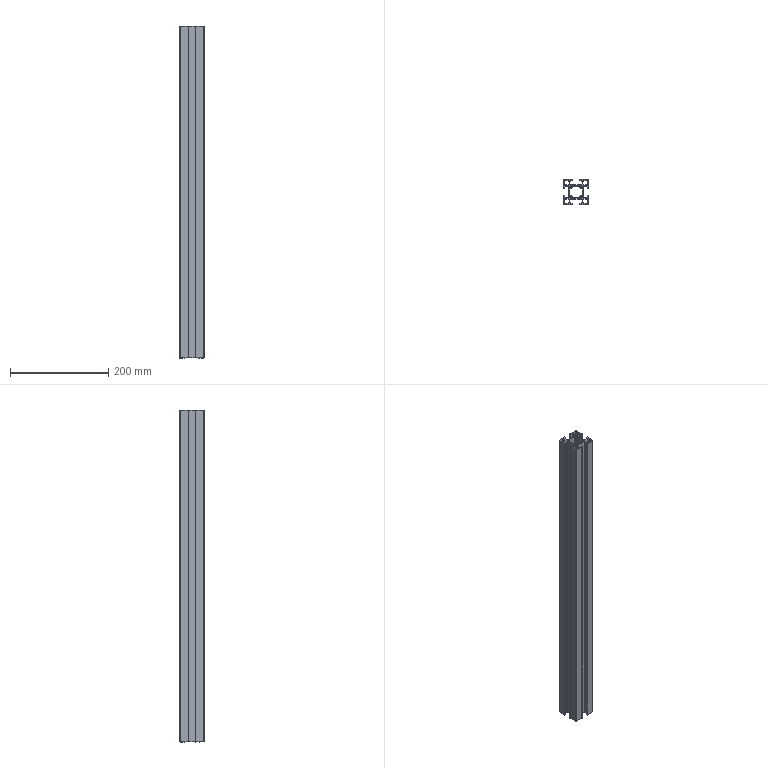Part | STEP file | DZZC_730mm | 1 solid | 142 faces | box 50 x 50 x 675 mm | volume 396557 mm3 | cylinder 84 | plane 58 | commonest cylinder face diameters 1 x24 4 x24 1.5 x16 3.7 x8 6.7 x8 2 x4